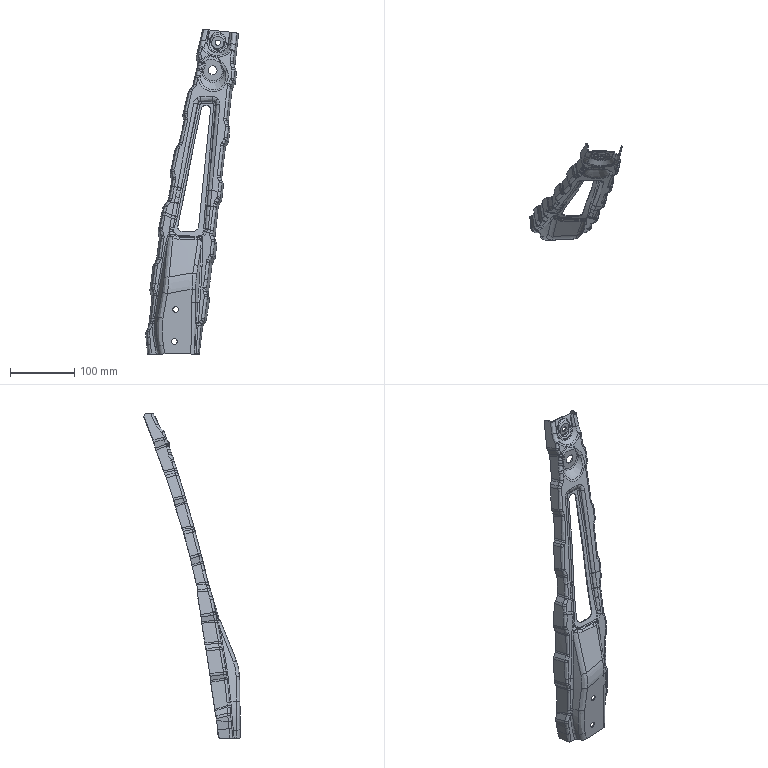Part | STEP file | FNA5401631 | 1 solid | 903 faces | box 144.102 x 149.837 x 505.997 mm | volume 84587 mm3 | spline 734 | cylinder 62 | plane 57 | other 44 | sphere 6 | commonest cylinder face diameters 13 x10 16 x10 9 x9 6 x7 10 x3 14 x3